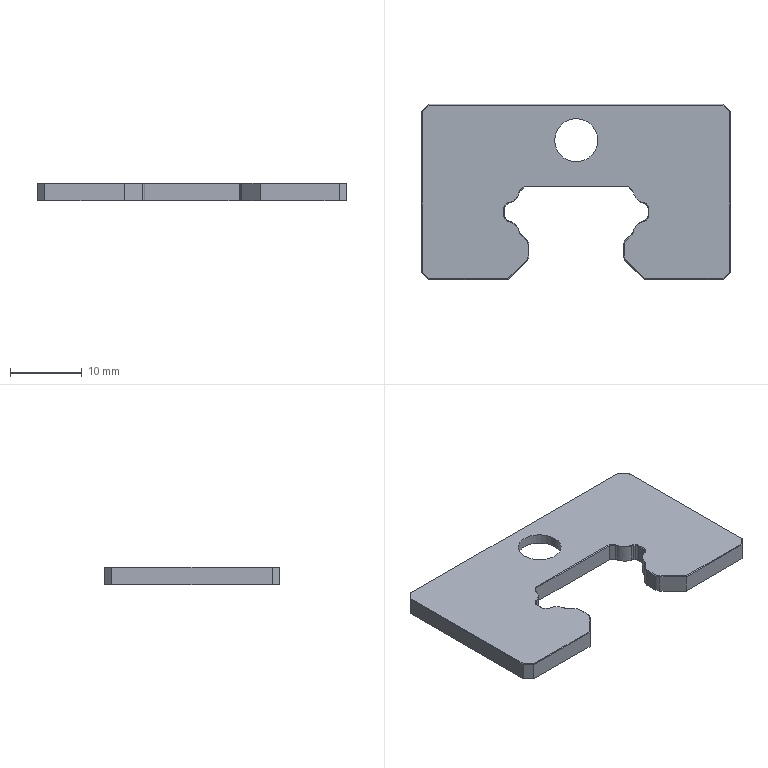Part | STEP file | PART1AAA^SUB1AA_P-008243 | 1 solid | 100 faces | box 43 x 24.4 x 2.5 mm | volume 1956 mm3 | plane 57 | cylinder 23 | cone 20 | commonest cylinder face diameters 1 x12 2 x4 4.06 x4 6 x2 10 x1